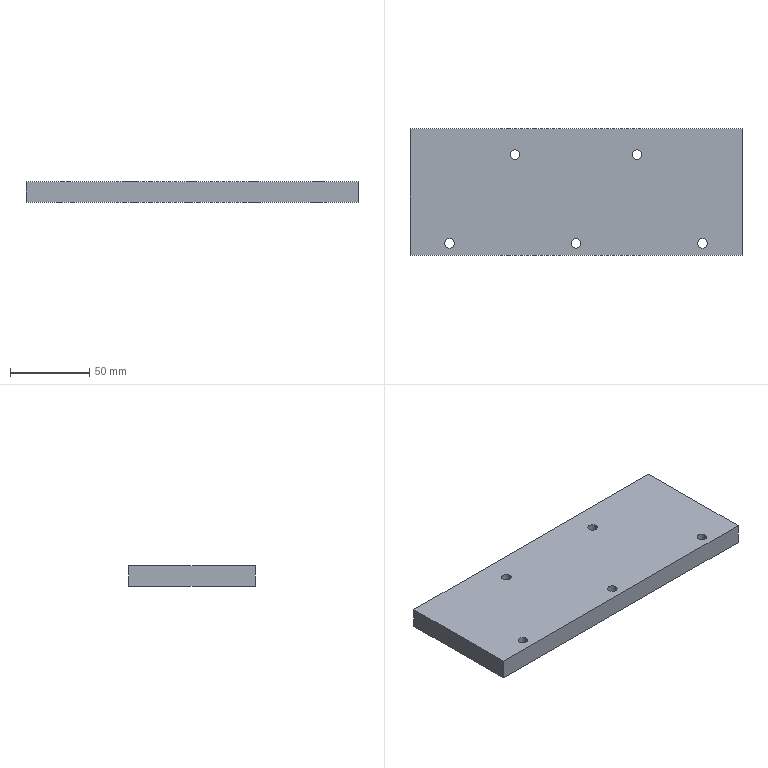Part | SolidWorks | features Cut 4, 3DProfileFeature 2, HoleWzd 2, Extrusion 1 | 1 solid | 39 faces | box 210 x 80 x 13 mm | volume 214445 mm3 | cylinder 24 | plane 11 | cone 4 | commonest cylinder face diameters 6 x10 10 x10 5 x4
STEP:
#1=CARTESIAN_POINT('',(90.,28.,9.));
#2=VERTEX_POINT('',#1);
#3=CARTESIAN_POINT('',(90.,28.,4.));
#4=VERTEX_POINT('',#3);
#5=CARTESIAN_POINT('',(90.,28.,6.5));
#6=DIRECTION('',(1.,0.,0.));
#7=DIRECTION('',(0.,0.,-1.));
#8=AXIS2_PLACEMENT_3D('',#5,#6,#7);
#9=CIRCLE('',#8,2.5);
#10=EDGE_CURVE('',#2,#4,#9,.T.);
#11=ORIENTED_EDGE('',*,*,#10,.F.);
#12=CARTESIAN_POINT('',(105.,28.,9.));
#13=VERTEX_POINT('',#12);
#14=CARTESIAN_POINT('',(105.,28.,9.));
#15=DIRECTION('',(1.,0.,0.));
#16=VECTOR('',#15,1000.);
#17=LINE('',#14,#16);
#18=EDGE_CURVE('',#2,#13,#17,.T.);
#19=ORIENTED_EDGE('',*,*,#18,.T.);
#20=CARTESIAN_POINT('',(105.,28.,4.));
#21=VERTEX_POINT('',#20);
#22=CARTESIAN_POINT('',(105.,28.,6.5));
#23=DIRECTION('',(1.,0.,0.));
#24=DIRECTION('',(0.,0.,-1.));
#25=AXIS2_PLACEMENT_3D('',#22,#23,#24);
#26=CIRCLE('',#25,2.5);
#27=EDGE_CURVE('',#13,#21,#26,.T.);
#28=ORIENTED_EDGE('',*,*,#27,.T.);
#29=CARTESIAN_POINT('',(105.,28.,4.));
#30=DIRECTION('',(1.,0.,0.));
#31=VECTOR('',#30,1000.);
#32=LINE('',#29,#31);
#33=EDGE_CURVE('',#4,#21,#32,.T.);
#34=ORIENTED_EDGE('',*,*,#33,.F.);
#35=EDGE_LOOP('',(#11,#19,#28,#34));
#36=FACE_OUTER_BOUND('',#35,.T.);
#37=CARTESIAN_POINT('',(105.,28.,6.5));
#38=DIRECTION('',(1.,0.,0.));
#39=DIRECTION('',(0.,0.,-1.));
#40=AXIS2_PLACEMENT_3D('',#37,#38,#39);
#41=CYLINDRICAL_SURFACE('',#40,2.5);
#42=ADVANCED_FACE('',(#36),#41,.F.);
#43=CARTESIAN_POINT('',(88.498,28.,6.5));
#44=VERTEX_POINT('',#43);
#45=CARTESIAN_POINT('',(90.,28.,4.));
#46=DIRECTION('',(0.515,0.,-0.8572));
#47=VECTOR('',#46,1000.);
#48=LINE('',#45,#47);
#49=EDGE_CURVE('',#44,#4,#48,.T.);
#50=ORIENTED_EDGE('',*,*,#49,.F.);
#51=CARTESIAN_POINT('',(90.,28.,9.));
#52=DIRECTION('',(0.515,0.,0.8572));
#53=VECTOR('',#52,1000.);
#54=LINE('',#51,#53);
#55=EDGE_CURVE('',#44,#2,#54,.T.);
#56=ORIENTED_EDGE('',*,*,#55,.T.);
#57=ORIENTED_EDGE('',*,*,#10,.T.);
#58=EDGE_LOOP('',(#50,#56,#57));
#59=FACE_OUTER_BOUND('',#58,.T.);
#60=CARTESIAN_POINT('',(90.,28.,6.5));
#61=DIRECTION('',(1.,0.,0.));
#62=DIRECTION('',(0.,0.,-1.));
#63=AXIS2_PLACEMENT_3D('',#60,#61,#62);
#64=CONICAL_SURFACE('',#63,2.5,1.03);
#65=ADVANCED_FACE('',(#59),#64,.F.);
#66=CARTESIAN_POINT('',(-83.,-32.5,13.));
#67=VERTEX_POINT('',#66);
#68=CARTESIAN_POINT('',(-77.,-32.5,13.));
#69=VERTEX_POINT('',#68);
#70=CARTESIAN_POINT('',(-80.,-32.5,13.));
#71=DIRECTION('',(0.,0.,1.));
#72=DIRECTION('',(-1.,0.,0.));
#73=AXIS2_PLACEMENT_3D('',#70,#71,#72);
#74=CIRCLE('',#73,3.);
#75=EDGE_CURVE('',#67,#69,#74,.T.);
#76=ORIENTED_EDGE('',*,*,#75,.T.);
#77=CARTESIAN_POINT('',(-77.,-32.5,6.));
#78=VERTEX_POINT('',#77);
#79=CARTESIAN_POINT('',(-77.,-32.5,13.001));
#80=DIRECTION('',(0.,0.,-1.));
#81=VECTOR('',#80,1000.);
#82=LINE('',#79,#81);
#83=EDGE_CURVE('',#69,#78,#82,.T.);
#84=ORIENTED_EDGE('',*,*,#83,.T.);
#85=CARTESIAN_POINT('',(-83.,-32.5,6.));
#86=VERTEX_POINT('',#85);
#87=CARTESIAN_POINT('',(-80.,-32.5,6.));
#88=DIRECTION('',(0.,0.,1.));
#89=DIRECTION('',(-1.,0.,0.));
#90=AXIS2_PLACEMENT_3D('',#87,#88,#89);
#91=CIRCLE('',#90,3.);
#92=EDGE_CURVE('',#86,#78,#91,.T.);
#93=ORIENTED_EDGE('',*,*,#92,.F.);
#94=CARTESIAN_POINT('',(-83.,-32.5,13.001));
#95=DIRECTION('',(0.,0.,-1.));
#96=VECTOR('',#95,1000.);
#97=LINE('',#94,#96);
#98=EDGE_CURVE('',#67,#86,#97,.T.);
#99=ORIENTED_EDGE('',*,*,#98,.F.);
#100=EDGE_LOOP('',(#76,#84,#93,#99));
#101=FACE_OUTER_BOUND('',#100,.T.);
#102=CARTESIAN_POINT('',(-80.,-32.5,13.001));
#103=DIRECTION('',(0.,0.,-1.));
#104=DIRECTION('',(-1.,0.,0.));
#105=AXIS2_PLACEMENT_3D('',#102,#103,#104);
#106=CYLINDRICAL_SURFACE('',#105,3.);
#107=ADVANCED_FACE('',(#101),#106,.F.);
#108=CARTESIAN_POINT('',(-3.,-32.5,13.));
#109=VERTEX_POINT('',#108);
#110=CARTESIAN_POINT('',(3.,-32.5,13.));
#111=VERTEX_POINT('',#110);
#112=CARTESIAN_POINT('',(0.,-32.5,13.));
#113=DIRECTION('',(0.,0.,1.));
#114=DIRECTION('',(-1.,0.,0.));
#115=AXIS2_PLACEMENT_3D('',#112,#113,#114);
#116=CIRCLE('',#115,3.);
#117=EDGE_CURVE('',#109,#111,#116,.T.);
#118=ORIENTED_EDGE('',*,*,#117,.T.);
#119=CARTESIAN_POINT('',(3.,-32.5,6.));
#120=VERTEX_POINT('',#119);
#121=CARTESIAN_POINT('',(3.,-32.5,13.001));
#122=DIRECTION('',(0.,0.,-1.));
#123=VECTOR('',#122,1000.);
#124=LINE('',#121,#123);
#125=EDGE_CURVE('',#111,#120,#124,.T.);
#126=ORIENTED_EDGE('',*,*,#125,.T.);
#127=CARTESIAN_POINT('',(-3.,-32.5,6.));
#128=VERTEX_POINT('',#127);
#129=CARTESIAN_POINT('',(0.,-32.5,6.));
#130=DIRECTION('',(0.,0.,1.));
#131=DIRECTION('',(-1.,0.,0.));
#132=AXIS2_PLACEMENT_3D('',#129,#130,#131);
#133=CIRCLE('',#132,3.);
#134=EDGE_CURVE('',#128,#120,#133,.T.);
#135=ORIENTED_EDGE('',*,*,#134,.F.);
#136=CARTESIAN_POINT('',(-3.,-32.5,13.001));
#137=DIRECTION('',(0.,0.,-1.));
#138=VECTOR('',#137,1000.);
#139=LINE('',#136,#138);
#140=EDGE_CURVE('',#109,#128,#139,.T.);
#141=ORIENTED_EDGE('',*,*,#140,.F.);
#142=EDGE_LOOP('',(#118,#126,#135,#141));
#143=FACE_OUTER_BOUND('',#142,.T.);
#144=CARTESIAN_POINT('',(0.,-32.5,13.001));
#145=DIRECTION('',(0.,0.,-1.));
#146=DIRECTION('',(-1.,0.,0.));
#147=AXIS2_PLACEMENT_3D('',#144,#145,#146);
#148=CYLINDRICAL_SURFACE('',#147,3.);
#149=ADVANCED_FACE('',(#143),#148,.F.);
#150=CARTESIAN_POINT('',(77.,-32.5,13.));
#151=VERTEX_POINT('',#150);
#152=CARTESIAN_POINT('',(83.,-32.5,13.));
#153=VERTEX_POINT('',#152);
#154=CARTESIAN_POINT('',(80.,-32.5,13.));
#155=DIRECTION('',(0.,0.,1.));
#156=DIRECTION('',(-1.,0.,0.));
#157=AXIS2_PLACEMENT_3D('',#154,#155,#156);
#158=CIRCLE('',#157,3.);
#159=EDGE_CURVE('',#151,#153,#158,.T.);
#160=ORIENTED_EDGE('',*,*,#159,.T.);
#161=CARTESIAN_POINT('',(83.,-32.5,6.));
#162=VERTEX_POINT('',#161);
#163=CARTESIAN_POINT('',(83.,-32.5,13.001));
#164=DIRECTION('',(0.,0.,-1.));
#165=VECTOR('',#164,1000.);
#166=LINE('',#163,#165);
#167=EDGE_CURVE('',#153,#162,#166,.T.);
#168=ORIENTED_EDGE('',*,*,#167,.T.);
#169=CARTESIAN_POINT('',(77.,-32.5,6.));
#170=VERTEX_POINT('',#169);
#171=CARTESIAN_POINT('',(80.,-32.5,6.));
#172=DIRECTION('',(0.,0.,1.));
#173=DIRECTION('',(-1.,0.,0.));
#174=AXIS2_PLACEMENT_3D('',#171,#172,#173);
#175=CIRCLE('',#174,3.);
#176=EDGE_CURVE('',#170,#162,#175,.T.);
#177=ORIENTED_EDGE('',*,*,#176,.F.);
#178=CARTESIAN_POINT('',(77.,-32.5,13.001));
#179=DIRECTION('',(0.,0.,-1.));
#180=VECTOR('',#179,1000.);
#181=LINE('',#178,#180);
#182=EDGE_CURVE('',#151,#170,#181,.T.);
#183=ORIENTED_EDGE('',*,*,#182,.F.);
#184=EDGE_LOOP('',(#160,#168,#177,#183));
#185=FACE_OUTER_BOUND('',#184,.T.);
#186=CARTESIAN_POINT('',(80.,-32.5,13.001));
#187=DIRECTION('',(0.,0.,-1.));
#188=DIRECTION('',(-1.,0.,0.));
#189=AXIS2_PLACEMENT_3D('',#186,#187,#188);
#190=CYLINDRICAL_SURFACE('',#189,3.);
#191=ADVANCED_FACE('',(#185),#190,.F.);
#192=CARTESIAN_POINT('',(5.,-32.5,6.));
#193=VERTEX_POINT('',#192);
#194=CARTESIAN_POINT('',(-5.,-32.5,6.));
#195=VERTEX_POINT('',#194);
#196=CARTESIAN_POINT('',(0.,-32.5,6.));
#197=DIRECTION('',(0.,0.,-1.));
#198=DIRECTION('',(-1.,0.,0.));
#199=AXIS2_PLACEMENT_3D('',#196,#197,#198);
#200=CIRCLE('',#199,5.);
#201=EDGE_CURVE('',#193,#195,#200,.T.);
#202=ORIENTED_EDGE('',*,*,#201,.F.);
#203=CARTESIAN_POINT('',(5.,-32.5,0.));
#204=VERTEX_POINT('',#203);
#205=CARTESIAN_POINT('',(5.,-32.5,6.));
#206=DIRECTION('',(0.,0.,-1.));
#207=VECTOR('',#206,1000.);
#208=LINE('',#205,#207);
#209=EDGE_CURVE('',#193,#204,#208,.T.);
#210=ORIENTED_EDGE('',*,*,#209,.T.);
#211=CARTESIAN_POINT('',(-5.,-32.5,0.));
#212=VERTEX_POINT('',#211);
#213=CARTESIAN_POINT('',(0.,-32.5,0.));
#214=DIRECTION('',(0.,0.,-1.));
#215=DIRECTION('',(-1.,0.,0.));
#216=AXIS2_PLACEMENT_3D('',#213,#214,#215);
#217=CIRCLE('',#216,5.);
#218=EDGE_CURVE('',#204,#212,#217,.T.);
#219=ORIENTED_EDGE('',*,*,#218,.T.);
#220=CARTESIAN_POINT('',(-5.,-32.5,6.));
#221=DIRECTION('',(0.,0.,-1.));
#222=VECTOR('',#221,1000.);
#223=LINE('',#220,#222);
#224=EDGE_CURVE('',#195,#212,#223,.T.);
#225=ORIENTED_EDGE('',*,*,#224,.F.);
#226=EDGE_LOOP('',(#202,#210,#219,#225));
#227=FACE_OUTER_BOUND('',#226,.T.);
#228=CARTESIAN_POINT('',(0.,-32.5,6.));
#229=DIRECTION('',(0.,0.,-1.));
#230=DIRECTION('',(-1.,0.,0.));
#231=AXIS2_PLACEMENT_3D('',#228,#229,#230);
#232=CYLINDRICAL_SURFACE('',#231,5.);
#233=ADVANCED_FACE('',(#227),#232,.F.);
#234=CARTESIAN_POINT('',(-75.,-32.5,6.));
#235=VERTEX_POINT('',#234);
#236=CARTESIAN_POINT('',(-85.,-32.5,6.));
#237=VERTEX_POINT('',#236);
#238=CARTESIAN_POINT('',(-80.,-32.5,6.));
#239=DIRECTION('',(0.,0.,-1.));
#240=DIRECTION('',(-1.,0.,0.));
#241=AXIS2_PLACEMENT_3D('',#238,#239,#240);
#242=CIRCLE('',#241,5.);
#243=EDGE_CURVE('',#235,#237,#242,.T.);
#244=ORIENTED_EDGE('',*,*,#243,.F.);
#245=CARTESIAN_POINT('',(-75.,-32.5,0.));
#246=VERTEX_POINT('',#245);
#247=CARTESIAN_POINT('',(-75.,-32.5,6.));
#248=DIRECTION('',(0.,0.,-1.));
#249=VECTOR('',#248,1000.);
#250=LINE('',#247,#249);
#251=EDGE_CURVE('',#235,#246,#250,.T.);
#252=ORIENTED_EDGE('',*,*,#251,.T.);
#253=CARTESIAN_POINT('',(-85.,-32.5,0.));
#254=VERTEX_POINT('',#253);
#255=CARTESIAN_POINT('',(-80.,-32.5,0.));
#256=DIRECTION('',(0.,0.,-1.));
#257=DIRECTION('',(-1.,0.,0.));
#258=AXIS2_PLACEMENT_3D('',#255,#256,#257);
#259=CIRCLE('',#258,5.);
#260=EDGE_CURVE('',#246,#254,#259,.T.);
#261=ORIENTED_EDGE('',*,*,#260,.T.);
#262=CARTESIAN_POINT('',(-85.,-32.5,6.));
#263=DIRECTION('',(0.,0.,-1.));
#264=VECTOR('',#263,1000.);
#265=LINE('',#262,#264);
#266=EDGE_CURVE('',#237,#254,#265,.T.);
#267=ORIENTED_EDGE('',*,*,#266,.F.);
#268=EDGE_LOOP('',(#244,#252,#261,#267));
#269=FACE_OUTER_BOUND('',#268,.T.);
#270=CARTESIAN_POINT('',(-80.,-32.5,6.));
#271=DIRECTION('',(0.,0.,-1.));
#272=DIRECTION('',(-1.,0.,0.));
#273=AXIS2_PLACEMENT_3D('',#270,#271,#272);
#274=CYLINDRICAL_SURFACE('',#273,5.);
#275=ADVANCED_FACE('',(#269),#274,.F.);
#276=CARTESIAN_POINT('',(85.,-32.5,6.));
#277=VERTEX_POINT('',#276);
#278=CARTESIAN_POINT('',(75.,-32.5,6.));
#279=VERTEX_POINT('',#278);
#280=CARTESIAN_POINT('',(80.,-32.5,6.));
#281=DIRECTION('',(0.,0.,-1.));
#282=DIRECTION('',(-1.,0.,0.));
#283=AXIS2_PLACEMENT_3D('',#280,#281,#282);
#284=CIRCLE('',#283,5.);
#285=EDGE_CURVE('',#277,#279,#284,.T.);
#286=ORIENTED_EDGE('',*,*,#285,.F.);
#287=CARTESIAN_POINT('',(85.,-32.5,0.));
#288=VERTEX_POINT('',#287);
#289=CARTESIAN_POINT('',(85.,-32.5,6.));
#290=DIRECTION('',(0.,0.,-1.));
#291=VECTOR('',#290,1000.);
#292=LINE('',#289,#291);
#293=EDGE_CURVE('',#277,#288,#292,.T.);
#294=ORIENTED_EDGE('',*,*,#293,.T.);
#295=CARTESIAN_POINT('',(75.,-32.5,0.));
#296=VERTEX_POINT('',#295);
#297=CARTESIAN_POINT('',(80.,-32.5,0.));
#298=DIRECTION('',(0.,0.,-1.));
#299=DIRECTION('',(-1.,0.,0.));
#300=AXIS2_PLACEMENT_3D('',#297,#298,#299);
#301=CIRCLE('',#300,5.);
#302=EDGE_CURVE('',#288,#296,#301,.T.);
#303=ORIENTED_EDGE('',*,*,#302,.T.);
#304=CARTESIAN_POINT('',(75.,-32.5,6.));
#305=DIRECTION('',(0.,0.,-1.));
#306=VECTOR('',#305,1000.);
#307=LINE('',#304,#306);
#308=EDGE_CURVE('',#279,#296,#307,.T.);
#309=ORIENTED_EDGE('',*,*,#308,.F.);
#310=EDGE_LOOP('',(#286,#294,#303,#309));
#311=FACE_OUTER_BOUND('',#310,.T.);
#312=CARTESIAN_POINT('',(80.,-32.5,6.));
#313=DIRECTION('',(0.,0.,-1.));
#314=DIRECTION('',(-1.,0.,0.));
#315=AXIS2_PLACEMENT_3D('',#312,#313,#314);
#316=CYLINDRICAL_SURFACE('',#315,5.);
#317=ADVANCED_FACE('',(#311),#316,.F.);
#318=CARTESIAN_POINT('',(90.,-32.5,9.));
#319=VERTEX_POINT('',#318);
#320=CARTESIAN_POINT('',(90.,-32.5,4.));
#321=VERTEX_POINT('',#320);
#322=CARTESIAN_POINT('',(90.,-32.5,6.5));
#323=DIRECTION('',(1.,0.,0.));
#324=DIRECTION('',(0.,0.,-1.));
#325=AXIS2_PLACEMENT_3D('',#322,#323,#324);
#326=CIRCLE('',#325,2.5);
#327=EDGE_CURVE('',#319,#321,#326,.T.);
#328=ORIENTED_EDGE('',*,*,#327,.F.);
#329=CARTESIAN_POINT('',(105.,-32.5,9.));
#330=VERTEX_POINT('',#329);
#331=CARTESIAN_POINT('',(105.,-32.5,9.));
#332=DIRECTION('',(1.,0.,0.));
#333=VECTOR('',#332,1000.);
#334=LINE('',#331,#333);
#335=EDGE_CURVE('',#319,#330,#334,.T.);
#336=ORIENTED_EDGE('',*,*,#335,.T.);
#337=CARTESIAN_POINT('',(105.,-32.5,4.));
#338=VERTEX_POINT('',#337);
#339=CARTESIAN_POINT('',(105.,-32.5,6.5));
#340=DIRECTION('',(1.,0.,0.));
#341=DIRECTION('',(0.,0.,-1.));
#342=AXIS2_PLACEMENT_3D('',#339,#340,#341);
#343=CIRCLE('',#342,2.5);
#344=EDGE_CURVE('',#330,#338,#343,.T.);
#345=ORIENTED_EDGE('',*,*,#344,.T.);
#346=CARTESIAN_POINT('',(105.,-32.5,4.));
#347=DIRECTION('',(1.,0.,0.));
#348=VECTOR('',#347,1000.);
#349=LINE('',#346,#348);
#350=EDGE_CURVE('',#321,#338,#349,.T.);
#351=ORIENTED_EDGE('',*,*,#350,.F.);
#352=EDGE_LOOP('',(#328,#336,#345,#351));
#353=FACE_OUTER_BOUND('',#352,.T.);
#354=CARTESIAN_POINT('',(105.,-32.5,6.5));
#355=DIRECTION('',(1.,0.,0.));
#356=DIRECTION('',(0.,0.,-1.));
#357=AXIS2_PLACEMENT_3D('',#354,#355,#356);
#358=CYLINDRICAL_SURFACE('',#357,2.5);
#359=ADVANCED_FACE('',(#353),#358,.F.);
#360=CARTESIAN_POINT('',(88.498,-32.5,6.5));
#361=VERTEX_POINT('',#360);
#362=CARTESIAN_POINT('',(90.,-32.5,4.));
#363=DIRECTION('',(0.515,0.,-0.8572));
#364=VECTOR('',#363,1000.);
#365=LINE('',#362,#364);
#366=EDGE_CURVE('',#361,#321,#365,.T.);
#367=ORIENTED_EDGE('',*,*,#366,.F.);
#368=CARTESIAN_POINT('',(90.,-32.5,9.));
#369=DIRECTION('',(0.515,0.,0.8572));
#370=VECTOR('',#369,1000.);
#371=LINE('',#368,#370);
#372=EDGE_CURVE('',#361,#319,#371,.T.);
#373=ORIENTED_EDGE('',*,*,#372,.T.);
#374=ORIENTED_EDGE('',*,*,#327,.T.);
#375=EDGE_LOOP('',(#367,#373,#374));
#376=FACE_OUTER_BOUND('',#375,.T.);
#377=CARTESIAN_POINT('',(90.,-32.5,6.5));
#378=DIRECTION('',(1.,0.,0.));
#379=DIRECTION('',(0.,0.,-1.));
#380=AXIS2_PLACEMENT_3D('',#377,#378,#379);
#381=CONICAL_SURFACE('',#380,2.5,1.03);
#382=ADVANCED_FACE('',(#376),#381,.F.);
#383=CARTESIAN_POINT('',(-41.548,23.617,13.));
#384=VERTEX_POINT('',#383);
#385=CARTESIAN_POINT('',(-35.548,23.617,13.));
#386=VERTEX_POINT('',#385);
#387=CARTESIAN_POINT('',(-38.548,23.617,13.));
#388=DIRECTION('',(0.,0.,1.));
#389=DIRECTION('',(-1.,0.,0.));
#390=AXIS2_PLACEMENT_3D('',#387,#388,#389);
#391=CIRCLE('',#390,3.);
#392=EDGE_CURVE('',#384,#386,#391,.T.);
#393=ORIENTED_EDGE('',*,*,#392,.T.);
#394=CARTESIAN_POINT('',(-35.548,23.617,6.));
#395=VERTEX_POINT('',#394);
#396=CARTESIAN_POINT('',(-35.548,23.617,13.001));
#397=DIRECTION('',(0.,0.,-1.));
#398=VECTOR('',#397,1000.);
#399=LINE('',#396,#398);
#400=EDGE_CURVE('',#386,#395,#399,.T.);
#401=ORIENTED_EDGE('',*,*,#400,.T.);
#402=CARTESIAN_POINT('',(-41.548,23.617,6.));
#403=VERTEX_POINT('',#402);
#404=CARTESIAN_POINT('',(-38.548,23.617,6.));
#405=DIRECTION('',(0.,0.,1.));
#406=DIRECTION('',(-1.,0.,0.));
#407=AXIS2_PLACEMENT_3D('',#404,#405,#406);
#408=CIRCLE('',#407,3.);
#409=EDGE_CURVE('',#403,#395,#408,.T.);
#410=ORIENTED_EDGE('',*,*,#409,.F.);
#411=CARTESIAN_POINT('',(-41.548,23.617,13.001));
#412=DIRECTION('',(0.,0.,-1.));
#413=VECTOR('',#412,1000.);
#414=LINE('',#411,#413);
#415=EDGE_CURVE('',#384,#403,#414,.T.);
#416=ORIENTED_EDGE('',*,*,#415,.F.);
#417=EDGE_LOOP('',(#393,#401,#410,#416));
#418=FACE_OUTER_BOUND('',#417,.T.);
#419=CARTESIAN_POINT('',(-38.548,23.617,13.001));
#420=DIRECTION('',(0.,0.,-1.));
#421=DIRECTION('',(-1.,0.,0.));
#422=AXIS2_PLACEMENT_3D('',#419,#420,#421);
#423=CYLINDRICAL_SURFACE('',#422,3.);
#424=ADVANCED_FACE('',(#418),#423,.F.);
#425=CARTESIAN_POINT('',(35.524,23.617,13.));
#426=VERTEX_POINT('',#425);
#427=CARTESIAN_POINT('',(41.524,23.617,13.));
#428=VERTEX_POINT('',#427);
#429=CARTESIAN_POINT('',(38.524,23.617,13.));
#430=DIRECTION('',(0.,0.,1.));
#431=DIRECTION('',(-1.,0.,0.));
#432=AXIS2_PLACEMENT_3D('',#429,#430,#431);
#433=CIRCLE('',#432,3.);
#434=EDGE_CURVE('',#426,#428,#433,.T.);
#435=ORIENTED_EDGE('',*,*,#434,.T.);
#436=CARTESIAN_POINT('',(41.524,23.617,6.));
#437=VERTEX_POINT('',#436);
#438=CARTESIAN_POINT('',(41.524,23.617,13.001));
#439=DIRECTION('',(0.,0.,-1.));
#440=VECTOR('',#439,1000.);
#441=LINE('',#438,#440);
#442=EDGE_CURVE('',#428,#437,#441,.T.);
#443=ORIENTED_EDGE('',*,*,#442,.T.);
#444=CARTESIAN_POINT('',(35.524,23.617,6.));
#445=VERTEX_POINT('',#444);
#446=CARTESIAN_POINT('',(38.524,23.617,6.));
#447=DIRECTION('',(0.,0.,1.));
#448=DIRECTION('',(-1.,0.,0.));
#449=AXIS2_PLACEMENT_3D('',#446,#447,#448);
#450=CIRCLE('',#449,3.);
#451=EDGE_CURVE('',#445,#437,#450,.T.);
#452=ORIENTED_EDGE('',*,*,#451,.F.);
#453=CARTESIAN_POINT('',(35.524,23.617,13.001));
#454=DIRECTION('',(0.,0.,-1.));
#455=VECTOR('',#454,1000.);
#456=LINE('',#453,#455);
#457=EDGE_CURVE('',#426,#445,#456,.T.);
#458=ORIENTED_EDGE('',*,*,#457,.F.);
#459=EDGE_LOOP('',(#435,#443,#452,#458));
#460=FACE_OUTER_BOUND('',#459,.T.);
#461=CARTESIAN_POINT('',(38.524,23.617,13.001));
#462=DIRECTION('',(0.,0.,-1.));
#463=DIRECTION('',(-1.,0.,0.));
#464=AXIS2_PLACEMENT_3D('',#461,#462,#463);
#465=CYLINDRICAL_SURFACE('',#464,3.);
#466=ADVANCED_FACE('',(#460),#465,.F.);
#467=CARTESIAN_POINT('',(-33.548,23.617,6.));
#468=VERTEX_POINT('',#467);
#469=CARTESIAN_POINT('',(-43.548,23.617,6.));
#470=VERTEX_POINT('',#469);
#471=CARTESIAN_POINT('',(-38.548,23.617,6.));
#472=DIRECTION('',(0.,0.,-1.));
#473=DIRECTION('',(-1.,0.,0.));
#474=AXIS2_PLACEMENT_3D('',#471,#472,#473);
#475=CIRCLE('',#474,5.);
#476=EDGE_CURVE('',#468,#470,#475,.T.);
#477=ORIENTED_EDGE('',*,*,#476,.F.);
#478=CARTESIAN_POINT('',(-33.548,23.617,0.));
#479=VERTEX_POINT('',#478);
#480=CARTESIAN_POINT('',(-33.548,23.617,6.));
#481=DIRECTION('',(0.,0.,-1.));
#482=VECTOR('',#481,1000.);
#483=LINE('',#480,#482);
#484=EDGE_CURVE('',#468,#479,#483,.T.);
#485=ORIENTED_EDGE('',*,*,#484,.T.);
#486=CARTESIAN_POINT('',(-43.548,23.617,0.));
#487=VERTEX_POINT('',#486);
#488=CARTESIAN_POINT('',(-38.548,23.617,0.));
#489=DIRECTION('',(0.,0.,-1.));
#490=DIRECTION('',(-1.,0.,0.));
#491=AXIS2_PLACEMENT_3D('',#488,#489,#490);
#492=CIRCLE('',#491,5.);
#493=EDGE_CURVE('',#479,#487,#492,.T.);
#494=ORIENTED_EDGE('',*,*,#493,.T.);
#495=CARTESIAN_POINT('',(-43.548,23.617,6.));
#496=DIRECTION('',(0.,0.,-1.));
#497=VECTOR('',#496,1000.);
#498=LINE('',#495,#497);
#499=EDGE_CURVE('',#470,#487,#498,.T.);
#500=ORIENTED_EDGE('',*,*,#499,.F.);
#501=EDGE_LOOP('',(#477,#485,#494,#500));
#502=FACE_OUTER_BOUND('',#501,.T.);
#503=CARTESIAN_POINT('',(-38.548,23.617,6.));
#504=DIRECTION('',(0.,0.,-1.));
#505=DIRECTION('',(-1.,0.,0.));
#506=AXIS2_PLACEMENT_3D('',#503,#504,#505);
#507=CYLINDRICAL_SURFACE('',#506,5.);
#508=ADVANCED_FACE('',(#502),#507,.F.);
#509=CARTESIAN_POINT('',(43.524,23.617,6.));
#510=VERTEX_POINT('',#509);
#511=CARTESIAN_POINT('',(33.524,23.617,6.));
#512=VERTEX_POINT('',#511);
#513=CARTESIAN_POINT('',(38.524,23.617,6.));
#514=DIRECTION('',(0.,0.,-1.));
#515=DIRECTION('',(-1.,0.,0.));
#516=AXIS2_PLACEMENT_3D('',#513,#514,#515);
#517=CIRCLE('',#516,5.);
#518=EDGE_CURVE('',#510,#512,#517,.T.);
#519=ORIENTED_EDGE('',*,*,#518,.F.);
#520=CARTESIAN_POINT('',(43.524,23.617,0.));
#521=VERTEX_POINT('',#520);
#522=CARTESIAN_POINT('',(43.524,23.617,6.));
#523=DIRECTION('',(0.,0.,-1.));
#524=VECTOR('',#523,1000.);
#525=LINE('',#522,#524);
#526=EDGE_CURVE('',#510,#521,#525,.T.);
#527=ORIENTED_EDGE('',*,*,#526,.T.);
#528=CARTESIAN_POINT('',(33.524,23.617,0.));
#529=VERTEX_POINT('',#528);
#530=CARTESIAN_POINT('',(38.524,23.617,0.));
#531=DIRECTION('',(0.,0.,-1.));
#532=DIRECTION('',(-1.,0.,0.));
#533=AXIS2_PLACEMENT_3D('',#530,#531,#532);
#534=CIRCLE('',#533,5.);
#535=EDGE_CURVE('',#521,#529,#534,.T.);
#536=ORIENTED_EDGE('',*,*,#535,.T.);
#537=CARTESIAN_POINT('',(33.524,23.617,6.));
#538=DIRECTION('',(0.,0.,-1.));
#539=VECTOR('',#538,1000.);
#540=LINE('',#537,#539);
#541=EDGE_CURVE('',#512,#529,#540,.T.);
#542=ORIENTED_EDGE('',*,*,#541,.F.);
#543=EDGE_LOOP('',(#519,#527,#536,#542));
#544=FACE_OUTER_BOUND('',#543,.T.);
#545=CARTESIAN_POINT('',(38.524,23.617,6.));
#546=DIRECTION('',(0.,0.,-1.));
#547=DIRECTION('',(-1.,0.,0.));
#548=AXIS2_PLACEMENT_3D('',#545,#546,#547);
#549=CYLINDRICAL_SURFACE('',#548,5.);
#550=ADVANCED_FACE('',(#544),#549,.F.);
#551=CARTESIAN_POINT('',(105.,28.,6.5));
#552=DIRECTION('',(1.,0.,0.));
#553=DIRECTION('',(0.,0.,-1.));
#554=AXIS2_PLACEMENT_3D('',#551,#552,#553);
#555=CIRCLE('',#554,2.5);
#556=EDGE_CURVE('',#21,#13,#555,.T.);
#557=ORIENTED_EDGE('',*,*,#556,.F.);
#558=ORIENTED_EDGE('',*,*,#27,.F.);
#559=EDGE_LOOP('',(#557,#558));
#560=FACE_BOUND('',#559,.T.);
#561=CARTESIAN_POINT('',(105.,-32.5,6.5));
#562=DIRECTION('',(1.,0.,0.));
#563=DIRECTION('',(0.,0.,-1.));
#564=AXIS2_PLACEMENT_3D('',#561,#562,#563);
#565=CIRCLE('',#564,2.5);
#566=EDGE_CURVE('',#338,#330,#565,.T.);
#567=ORIENTED_EDGE('',*,*,#566,.F.);
#568=ORIENTED_EDGE('',*,*,#344,.F.);
#569=EDGE_LOOP('',(#567,#568));
#570=FACE_BOUND('',#569,.T.);
#571=CARTESIAN_POINT('',(105.,-40.,0.));
#572=VERTEX_POINT('',#571);
#573=CARTESIAN_POINT('',(105.,40.,0.));
#574=VERTEX_POINT('',#573);
#575=CARTESIAN_POINT('',(105.,-40.,0.));
#576=DIRECTION('',(0.,1.,0.));
#577=VECTOR('',#576,1000.);
#578=LINE('',#575,#577);
#579=EDGE_CURVE('',#572,#574,#578,.T.);
#580=ORIENTED_EDGE('',*,*,#579,.T.);
#581=CARTESIAN_POINT('',(105.,40.,13.));
#582=VERTEX_POINT('',#581);
#583=CARTESIAN_POINT('',(105.,40.,13.));
#584=DIRECTION('',(0.,0.,-1.));
#585=VECTOR('',#584,1000.);
#586=LINE('',#583,#585);
#587=EDGE_CURVE('',#582,#574,#586,.T.);
#588=ORIENTED_EDGE('',*,*,#587,.F.);
#589=CARTESIAN_POINT('',(105.,-40.,13.));
#590=VERTEX_POINT('',#589);
#591=CARTESIAN_POINT('',(105.,-40.,13.));
#592=DIRECTION('',(0.,1.,0.));
#593=VECTOR('',#592,1000.);
#594=LINE('',#591,#593);
#595=EDGE_CURVE('',#590,#582,#594,.T.);
#596=ORIENTED_EDGE('',*,*,#595,.F.);
#597=CARTESIAN_POINT('',(105.,-40.,13.));
#598=DIRECTION('',(0.,0.,-1.));
#599=VECTOR('',#598,1000.);
#600=LINE('',#597,#599);
#601=EDGE_CURVE('',#590,#572,#600,.T.);
#602=ORIENTED_EDGE('',*,*,#601,.T.);
#603=EDGE_LOOP('',(#580,#588,#596,#602));
#604=FACE_OUTER_BOUND('',#603,.T.);
#605=CARTESIAN_POINT('',(105.,-40.,13.));
#606=DIRECTION('',(-1.,0.,0.));
#607=DIRECTION('',(0.,0.,1.));
#608=AXIS2_PLACEMENT_3D('',#605,#606,#607);
#609=PLANE('',#608);
#610=ADVANCED_FACE('',(#560,#570,#604),#609,.F.);
#611=CARTESIAN_POINT('',(-105.,40.,0.));
#612=VERTEX_POINT('',#611);
#613=CARTESIAN_POINT('',(-105.,40.,0.));
#614=DIRECTION('',(-1.,0.,0.));
#615=VECTOR('',#614,1000.);
#616=LINE('',#613,#615);
#617=EDGE_CURVE('',#574,#612,#616,.T.);
#618=ORIENTED_EDGE('',*,*,#617,.T.);
#619=CARTESIAN_POINT('',(-105.,40.,13.));
#620=VERTEX_POINT('',#619);
#621=CARTESIAN_POINT('',(-105.,40.,13.));
#622=DIRECTION('',(0.,0.,-1.));
#623=VECTOR('',#622,1000.);
#624=LINE('',#621,#623);
#625=EDGE_CURVE('',#620,#612,#624,.T.);
#626=ORIENTED_EDGE('',*,*,#625,.F.);
#627=CARTESIAN_POINT('',(-105.,40.,13.));
#628=DIRECTION('',(-1.,0.,0.));
#629=VECTOR('',#628,1000.);
#630=LINE('',#627,#629);
#631=EDGE_CURVE('',#582,#620,#630,.T.);
#632=ORIENTED_EDGE('',*,*,#631,.F.);
#633=ORIENTED_EDGE('',*,*,#587,.T.);
#634=EDGE_LOOP('',(#618,#626,#632,#633));
#635=FACE_OUTER_BOUND('',#634,.T.);
#636=CARTESIAN_POINT('',(-105.,40.,13.));
#637=DIRECTION('',(0.,-1.,0.));
#638=DIRECTION('',(0.,0.,-1.));
#639=AXIS2_PLACEMENT_3D('',#636,#637,#638);
#640=PLANE('',#639);
#641=ADVANCED_FACE('',(#635),#640,.F.);
#642=CARTESIAN_POINT('',(-105.,-40.,0.));
#643=VERTEX_POINT('',#642);
#644=CARTESIAN_POINT('',(-105.,-40.,0.));
#645=DIRECTION('',(0.,-1.,0.));
#646=VECTOR('',#645,1000.);
#647=LINE('',#644,#646);
#648=EDGE_CURVE('',#612,#643,#647,.T.);
#649=ORIENTED_EDGE('',*,*,#648,.T.);
#650=CARTESIAN_POINT('',(-105.,-40.,13.));
#651=VERTEX_POINT('',#650);
#652=CARTESIAN_POINT('',(-105.,-40.,13.));
#653=DIRECTION('',(0.,0.,-1.));
#654=VECTOR('',#653,1000.);
#655=LINE('',#652,#654);
#656=EDGE_CURVE('',#651,#643,#655,.T.);
#657=ORIENTED_EDGE('',*,*,#656,.F.);
#658=CARTESIAN_POINT('',(-105.,-40.,13.));
#659=DIRECTION('',(0.,-1.,0.));
#660=VECTOR('',#659,1000.);
#661=LINE('',#658,#660);
#662=EDGE_CURVE('',#620,#651,#661,.T.);
#663=ORIENTED_EDGE('',*,*,#662,.F.);
#664=ORIENTED_EDGE('',*,*,#625,.T.);
#665=EDGE_LOOP('',(#649,#657,#663,#664));
#666=FACE_OUTER_BOUND('',#665,.T.);
#667=CARTESIAN_POINT('',(-105.,-40.,13.));
#668=DIRECTION('',(1.,0.,0.));
#669=DIRECTION('',(0.,0.,-1.));
#670=AXIS2_PLACEMENT_3D('',#667,#668,#669);
#671=PLANE('',#670);
#672=ADVANCED_FACE('',(#666),#671,.F.);
#673=CARTESIAN_POINT('',(-105.,-40.,0.));
#674=DIRECTION('',(1.,0.,0.));
#675=VECTOR('',#674,1000.);
#676=LINE('',#673,#675);
#677=EDGE_CURVE('',#643,#572,#676,.T.);
#678=ORIENTED_EDGE('',*,*,#677,.T.);
#679=ORIENTED_EDGE('',*,*,#601,.F.);
#680=CARTESIAN_POINT('',(-105.,-40.,13.));
#681=DIRECTION('',(1.,0.,0.));
#682=VECTOR('',#681,1000.);
#683=LINE('',#680,#682);
#684=EDGE_CURVE('',#651,#590,#683,.T.);
#685=ORIENTED_EDGE('',*,*,#684,.F.);
#686=ORIENTED_EDGE('',*,*,#656,.T.);
#687=EDGE_LOOP('',(#678,#679,#685,#686));
#688=FACE_OUTER_BOUND('',#687,.T.);
#689=CARTESIAN_POINT('',(-105.,-40.,13.));
#690=DIRECTION('',(0.,1.,0.));
#691=DIRECTION('',(0.,0.,1.));
#692=AXIS2_PLACEMENT_3D('',#689,#690,#691);
#693=PLANE('',#692);
#694=ADVANCED_FACE('',(#688),#693,.F.);
#695=ORIENTED_EDGE('',*,*,#75,.F.);
#696=CARTESIAN_POINT('',(-80.,-32.5,13.));
#697=DIRECTION('',(0.,0.,1.));
#698=DIRECTION('',(-1.,0.,0.));
#699=AXIS2_PLACEMENT_3D('',#696,#697,#698);
#700=CIRCLE('',#699,3.);
#701=EDGE_CURVE('',#69,#67,#700,.T.);
#702=ORIENTED_EDGE('',*,*,#701,.F.);
#703=EDGE_LOOP('',(#695,#702));
#704=FACE_BOUND('',#703,.T.);
#705=ORIENTED_EDGE('',*,*,#117,.F.);
#706=CARTESIAN_POINT('',(0.,-32.5,13.));
#707=DIRECTION('',(0.,0.,1.));
#708=DIRECTION('',(-1.,0.,0.));
#709=AXIS2_PLACEMENT_3D('',#706,#707,#708);
#710=CIRCLE('',#709,3.);
#711=EDGE_CURVE('',#111,#109,#710,.T.);
#712=ORIENTED_EDGE('',*,*,#711,.F.);
#713=EDGE_LOOP('',(#705,#712));
#714=FACE_BOUND('',#713,.T.);
#715=ORIENTED_EDGE('',*,*,#159,.F.);
#716=CARTESIAN_POINT('',(80.,-32.5,13.));
#717=DIRECTION('',(0.,0.,1.));
#718=DIRECTION('',(-1.,0.,0.));
#719=AXIS2_PLACEMENT_3D('',#716,#717,#718);
#720=CIRCLE('',#719,3.);
#721=EDGE_CURVE('',#153,#151,#720,.T.);
#722=ORIENTED_EDGE('',*,*,#721,.F.);
#723=EDGE_LOOP('',(#715,#722));
#724=FACE_BOUND('',#723,.T.);
#725=ORIENTED_EDGE('',*,*,#392,.F.);
#726=CARTESIAN_POINT('',(-38.548,23.617,13.));
#727=DIRECTION('',(0.,0.,1.));
#728=DIRECTION('',(-1.,0.,0.));
#729=AXIS2_PLACEMENT_3D('',#726,#727,#728);
#730=CIRCLE('',#729,3.);
#731=EDGE_CURVE('',#386,#384,#730,.T.);
#732=ORIENTED_EDGE('',*,*,#731,.F.);
#733=EDGE_LOOP('',(#725,#732));
#734=FACE_BOUND('',#733,.T.);
#735=ORIENTED_EDGE('',*,*,#434,.F.);
#736=CARTESIAN_POINT('',(38.524,23.617,13.));
#737=DIRECTION('',(0.,0.,1.));
#738=DIRECTION('',(-1.,0.,0.));
#739=AXIS2_PLACEMENT_3D('',#736,#737,#738);
#740=CIRCLE('',#739,3.);
#741=EDGE_CURVE('',#428,#426,#740,.T.);
#742=ORIENTED_EDGE('',*,*,#741,.F.);
#743=EDGE_LOOP('',(#735,#742));
#744=FACE_BOUND('',#743,.T.);
#745=ORIENTED_EDGE('',*,*,#595,.T.);
#746=ORIENTED_EDGE('',*,*,#631,.T.);
#747=ORIENTED_EDGE('',*,*,#662,.T.);
#748=ORIENTED_EDGE('',*,*,#684,.T.);
#749=EDGE_LOOP('',(#745,#746,#747,#748));
#750=FACE_OUTER_BOUND('',#749,.T.);
#751=CARTESIAN_POINT('',(0.,0.,13.));
#752=DIRECTION('',(0.,0.,-1.));
#753=DIRECTION('',(-1.,0.,0.));
#754=AXIS2_PLACEMENT_3D('',#751,#752,#753);
#755=PLANE('',#754);
#756=ADVANCED_FACE('',(#704,#714,#724,#734,#744,#750),#755,.F.);
#757=CARTESIAN_POINT('',(0.,-32.5,0.));
#758=DIRECTION('',(0.,0.,-1.));
#759=DIRECTION('',(-1.,0.,0.));
#760=AXIS2_PLACEMENT_3D('',#757,#758,#759);
#761=CIRCLE('',#760,5.);
#762=EDGE_CURVE('',#212,#204,#761,.T.);
#763=ORIENTED_EDGE('',*,*,#762,.F.);
#764=ORIENTED_EDGE('',*,*,#218,.F.);
#765=EDGE_LOOP('',(#763,#764));
#766=FACE_BOUND('',#765,.T.);
#767=CARTESIAN_POINT('',(-80.,-32.5,0.));
#768=DIRECTION('',(0.,0.,-1.));
#769=DIRECTION('',(-1.,0.,0.));
#770=AXIS2_PLACEMENT_3D('',#767,#768,#769);
#771=CIRCLE('',#770,5.);
#772=EDGE_CURVE('',#254,#246,#771,.T.);
#773=ORIENTED_EDGE('',*,*,#772,.F.);
#774=ORIENTED_EDGE('',*,*,#260,.F.);
#775=EDGE_LOOP('',(#773,#774));
#776=FACE_BOUND('',#775,.T.);
#777=CARTESIAN_POINT('',(80.,-32.5,0.));
#778=DIRECTION('',(0.,0.,-1.));
#779=DIRECTION('',(-1.,0.,0.));
#780=AXIS2_PLACEMENT_3D('',#777,#778,#779);
#781=CIRCLE('',#780,5.);
#782=EDGE_CURVE('',#296,#288,#781,.T.);
#783=ORIENTED_EDGE('',*,*,#782,.F.);
#784=ORIENTED_EDGE('',*,*,#302,.F.);
#785=EDGE_LOOP('',(#783,#784));
#786=FACE_BOUND('',#785,.T.);
#787=CARTESIAN_POINT('',(-38.548,23.617,0.));
#788=DIRECTION('',(0.,0.,-1.));
#789=DIRECTION('',(-1.,0.,0.));
#790=AXIS2_PLACEMENT_3D('',#787,#788,#789);
#791=CIRCLE('',#790,5.);
#792=EDGE_CURVE('',#487,#479,#791,.T.);
#793=ORIENTED_EDGE('',*,*,#792,.F.);
#794=ORIENTED_EDGE('',*,*,#493,.F.);
#795=EDGE_LOOP('',(#793,#794));
#796=FACE_BOUND('',#795,.T.);
#797=CARTESIAN_POINT('',(38.524,23.617,0.));
#798=DIRECTION('',(0.,0.,-1.));
#799=DIRECTION('',(-1.,0.,0.));
#800=AXIS2_PLACEMENT_3D('',#797,#798,#799);
#801=CIRCLE('',#800,5.);
#802=EDGE_CURVE('',#529,#521,#801,.T.);
#803=ORIENTED_EDGE('',*,*,#802,.F.);
#804=ORIENTED_EDGE('',*,*,#535,.F.);
#805=EDGE_LOOP('',(#803,#804));
#806=FACE_BOUND('',#805,.T.);
#807=ORIENTED_EDGE('',*,*,#579,.F.);
#808=ORIENTED_EDGE('',*,*,#677,.F.);
#809=ORIENTED_EDGE('',*,*,#648,.F.);
#810=ORIENTED_EDGE('',*,*,#617,.F.);
#811=EDGE_LOOP('',(#807,#808,#809,#810));
#812=FACE_OUTER_BOUND('',#811,.T.);
#813=CARTESIAN_POINT('',(0.,0.,0.));
#814=DIRECTION('',(0.,0.,-1.));
#815=DIRECTION('',(-1.,0.,0.));
#816=AXIS2_PLACEMENT_3D('',#813,#814,#815);
#817=PLANE('',#816);
#818=ADVANCED_FACE('',(#766,#776,#786,#796,#806,#812),#817,.T.);
#819=ORIENTED_EDGE('',*,*,#526,.F.);
#820=CARTESIAN_POINT('',(38.524,23.617,6.));
#821=DIRECTION('',(0.,0.,-1.));
#822=DIRECTION('',(-1.,0.,0.));
#823=AXIS2_PLACEMENT_3D('',#820,#821,#822);
#824=CIRCLE('',#823,5.);
#825=EDGE_CURVE('',#512,#510,#824,.T.);
#826=ORIENTED_EDGE('',*,*,#825,.F.);
#827=ORIENTED_EDGE('',*,*,#541,.T.);
#828=ORIENTED_EDGE('',*,*,#802,.T.);
#829=EDGE_LOOP('',(#819,#826,#827,#828));
#830=FACE_OUTER_BOUND('',#829,.T.);
#831=CARTESIAN_POINT('',(38.524,23.617,6.));
#832=DIRECTION('',(0.,0.,-1.));
#833=DIRECTION('',(-1.,0.,0.));
#834=AXIS2_PLACEMENT_3D('',#831,#832,#833);
#835=CYLINDRICAL_SURFACE('',#834,5.);
#836=ADVANCED_FACE('',(#830),#835,.F.);
#837=ORIENTED_EDGE('',*,*,#451,.T.);
#838=CARTESIAN_POINT('',(38.524,23.617,6.));
#839=DIRECTION('',(0.,0.,1.));
#840=DIRECTION('',(-1.,0.,0.));
#841=AXIS2_PLACEMENT_3D('',#838,#839,#840);
#842=CIRCLE('',#841,3.);
#843=EDGE_CURVE('',#437,#445,#842,.T.);
#844=ORIENTED_EDGE('',*,*,#843,.T.);
#845=EDGE_LOOP('',(#837,#844));
#846=FACE_BOUND('',#845,.T.);
#847=ORIENTED_EDGE('',*,*,#825,.T.);
#848=ORIENTED_EDGE('',*,*,#518,.T.);
#849=EDGE_LOOP('',(#847,#848));
#850=FACE_OUTER_BOUND('',#849,.T.);
#851=CARTESIAN_POINT('',(0.,0.,6.));
#852=DIRECTION('',(0.,0.,-1.));
#853=DIRECTION('',(-1.,0.,0.));
#854=AXIS2_PLACEMENT_3D('',#851,#852,#853);
#855=PLANE('',#854);
#856=ADVANCED_FACE('',(#846,#850),#855,.T.);
#857=ORIENTED_EDGE('',*,*,#484,.F.);
#858=CARTESIAN_POINT('',(-38.548,23.617,6.));
#859=DIRECTION('',(0.,0.,-1.));
#860=DIRECTION('',(-1.,0.,0.));
#861=AXIS2_PLACEMENT_3D('',#858,#859,#860);
#862=CIRCLE('',#861,5.);
#863=EDGE_CURVE('',#470,#468,#862,.T.);
#864=ORIENTED_EDGE('',*,*,#863,.F.);
#865=ORIENTED_EDGE('',*,*,#499,.T.);
#866=ORIENTED_EDGE('',*,*,#792,.T.);
#867=EDGE_LOOP('',(#857,#864,#865,#866));
#868=FACE_OUTER_BOUND('',#867,.T.);
#869=CARTESIAN_POINT('',(-38.548,23.617,6.));
#870=DIRECTION('',(0.,0.,-1.));
#871=DIRECTION('',(-1.,0.,0.));
#872=AXIS2_PLACEMENT_3D('',#869,#870,#871);
#873=CYLINDRICAL_SURFACE('',#872,5.);
#874=ADVANCED_FACE('',(#868),#873,.F.);
#875=ORIENTED_EDGE('',*,*,#409,.T.);
#876=CARTESIAN_POINT('',(-38.548,23.617,6.));
#877=DIRECTION('',(0.,0.,1.));
#878=DIRECTION('',(-1.,0.,0.));
#879=AXIS2_PLACEMENT_3D('',#876,#877,#878);
#880=CIRCLE('',#879,3.);
#881=EDGE_CURVE('',#395,#403,#880,.T.);
#882=ORIENTED_EDGE('',*,*,#881,.T.);
#883=EDGE_LOOP('',(#875,#882));
#884=FACE_BOUND('',#883,.T.);
#885=ORIENTED_EDGE('',*,*,#863,.T.);
#886=ORIENTED_EDGE('',*,*,#476,.T.);
#887=EDGE_LOOP('',(#885,#886));
#888=FACE_OUTER_BOUND('',#887,.T.);
#889=CARTESIAN_POINT('',(0.,0.,6.));
#890=DIRECTION('',(0.,0.,-1.));
#891=DIRECTION('',(-1.,0.,0.));
#892=AXIS2_PLACEMENT_3D('',#889,#890,#891);
#893=PLANE('',#892);
#894=ADVANCED_FACE('',(#884,#888),#893,.T.);
#895=ORIENTED_EDGE('',*,*,#442,.F.);
#896=ORIENTED_EDGE('',*,*,#741,.T.);
#897=ORIENTED_EDGE('',*,*,#457,.T.);
#898=ORIENTED_EDGE('',*,*,#843,.F.);
#899=EDGE_LOOP('',(#895,#896,#897,#898));
#900=FACE_OUTER_BOUND('',#899,.T.);
#901=CARTESIAN_POINT('',(38.524,23.617,13.001));
#902=DIRECTION('',(0.,0.,-1.));
#903=DIRECTION('',(-1.,0.,0.));
#904=AXIS2_PLACEMENT_3D('',#901,#902,#903);
#905=CYLINDRICAL_SURFACE('',#904,3.);
#906=ADVANCED_FACE('',(#900),#905,.F.);
#907=ORIENTED_EDGE('',*,*,#400,.F.);
#908=ORIENTED_EDGE('',*,*,#731,.T.);
#909=ORIENTED_EDGE('',*,*,#415,.T.);
#910=ORIENTED_EDGE('',*,*,#881,.F.);
#911=EDGE_LOOP('',(#907,#908,#909,#910));
#912=FACE_OUTER_BOUND('',#911,.T.);
#913=CARTESIAN_POINT('',(-38.548,23.617,13.001));
#914=DIRECTION('',(0.,0.,-1.));
#915=DIRECTION('',(-1.,0.,0.));
#916=AXIS2_PLACEMENT_3D('',#913,#914,#915);
#917=CYLINDRICAL_SURFACE('',#916,3.);
#918=ADVANCED_FACE('',(#912),#917,.F.);
#919=ORIENTED_EDGE('',*,*,#372,.F.);
#920=ORIENTED_EDGE('',*,*,#366,.T.);
#921=CARTESIAN_POINT('',(90.,-32.5,6.5));
#922=DIRECTION('',(1.,0.,0.));
#923=DIRECTION('',(0.,0.,-1.));
#924=AXIS2_PLACEMENT_3D('',#921,#922,#923);
#925=CIRCLE('',#924,2.5);
#926=EDGE_CURVE('',#321,#319,#925,.T.);
#927=ORIENTED_EDGE('',*,*,#926,.T.);
#928=EDGE_LOOP('',(#919,#920,#927));
#929=FACE_OUTER_BOUND('',#928,.T.);
#930=CARTESIAN_POINT('',(90.,-32.5,6.5));
#931=DIRECTION('',(1.,0.,0.));
#932=DIRECTION('',(0.,0.,-1.));
#933=AXIS2_PLACEMENT_3D('',#930,#931,#932);
#934=CONICAL_SURFACE('',#933,2.5,1.03);
#935=ADVANCED_FACE('',(#929),#934,.F.);
#936=ORIENTED_EDGE('',*,*,#335,.F.);
#937=ORIENTED_EDGE('',*,*,#926,.F.);
#938=ORIENTED_EDGE('',*,*,#350,.T.);
#939=ORIENTED_EDGE('',*,*,#566,.T.);
#940=EDGE_LOOP('',(#936,#937,#938,#939));
#941=FACE_OUTER_BOUND('',#940,.T.);
#942=CARTESIAN_POINT('',(105.,-32.5,6.5));
#943=DIRECTION('',(1.,0.,0.));
#944=DIRECTION('',(0.,0.,-1.));
#945=AXIS2_PLACEMENT_3D('',#942,#943,#944);
#946=CYLINDRICAL_SURFACE('',#945,2.5);
#947=ADVANCED_FACE('',(#941),#946,.F.);
#948=ORIENTED_EDGE('',*,*,#293,.F.);
#949=CARTESIAN_POINT('',(80.,-32.5,6.));
#950=DIRECTION('',(0.,0.,-1.));
#951=DIRECTION('',(-1.,0.,0.));
#952=AXIS2_PLACEMENT_3D('',#949,#950,#951);
#953=CIRCLE('',#952,5.);
#954=EDGE_CURVE('',#279,#277,#953,.T.);
#955=ORIENTED_EDGE('',*,*,#954,.F.);
#956=ORIENTED_EDGE('',*,*,#308,.T.);
#957=ORIENTED_EDGE('',*,*,#782,.T.);
#958=EDGE_LOOP('',(#948,#955,#956,#957));
#959=FACE_OUTER_BOUND('',#958,.T.);
#960=CARTESIAN_POINT('',(80.,-32.5,6.));
#961=DIRECTION('',(0.,0.,-1.));
#962=DIRECTION('',(-1.,0.,0.));
#963=AXIS2_PLACEMENT_3D('',#960,#961,#962);
#964=CYLINDRICAL_SURFACE('',#963,5.);
#965=ADVANCED_FACE('',(#959),#964,.F.);
#966=ORIENTED_EDGE('',*,*,#176,.T.);
#967=CARTESIAN_POINT('',(80.,-32.5,6.));
#968=DIRECTION('',(0.,0.,1.));
#969=DIRECTION('',(-1.,0.,0.));
#970=AXIS2_PLACEMENT_3D('',#967,#968,#969);
#971=CIRCLE('',#970,3.);
#972=EDGE_CURVE('',#162,#170,#971,.T.);
#973=ORIENTED_EDGE('',*,*,#972,.T.);
#974=EDGE_LOOP('',(#966,#973));
#975=FACE_BOUND('',#974,.T.);
#976=ORIENTED_EDGE('',*,*,#954,.T.);
#977=ORIENTED_EDGE('',*,*,#285,.T.);
#978=EDGE_LOOP('',(#976,#977));
#979=FACE_OUTER_BOUND('',#978,.T.);
#980=CARTESIAN_POINT('',(0.,0.,6.));
#981=DIRECTION('',(0.,0.,-1.));
#982=DIRECTION('',(-1.,0.,0.));
#983=AXIS2_PLACEMENT_3D('',#980,#981,#982);
#984=PLANE('',#983);
#985=ADVANCED_FACE('',(#975,#979),#984,.T.);
#986=ORIENTED_EDGE('',*,*,#251,.F.);
#987=CARTESIAN_POINT('',(-80.,-32.5,6.));
#988=DIRECTION('',(0.,0.,-1.));
#989=DIRECTION('',(-1.,0.,0.));
#990=AXIS2_PLACEMENT_3D('',#987,#988,#989);
#991=CIRCLE('',#990,5.);
#992=EDGE_CURVE('',#237,#235,#991,.T.);
#993=ORIENTED_EDGE('',*,*,#992,.F.);
#994=ORIENTED_EDGE('',*,*,#266,.T.);
#995=ORIENTED_EDGE('',*,*,#772,.T.);
#996=EDGE_LOOP('',(#986,#993,#994,#995));
#997=FACE_OUTER_BOUND('',#996,.T.);
#998=CARTESIAN_POINT('',(-80.,-32.5,6.));
#999=DIRECTION('',(0.,0.,-1.));
#1000=DIRECTION('',(-1.,0.,0.));
#1001=AXIS2_PLACEMENT_3D('',#998,#999,#1000);
#1002=CYLINDRICAL_SURFACE('',#1001,5.);
#1003=ADVANCED_FACE('',(#997),#1002,.F.);
#1004=ORIENTED_EDGE('',*,*,#92,.T.);
#1005=CARTESIAN_POINT('',(-80.,-32.5,6.));
#1006=DIRECTION('',(0.,0.,1.));
#1007=DIRECTION('',(-1.,0.,0.));
#1008=AXIS2_PLACEMENT_3D('',#1005,#1006,#1007);
#1009=CIRCLE('',#1008,3.);
#1010=EDGE_CURVE('',#78,#86,#1009,.T.);
#1011=ORIENTED_EDGE('',*,*,#1010,.T.);
#1012=EDGE_LOOP('',(#1004,#1011));
#1013=FACE_BOUND('',#1012,.T.);
#1014=ORIENTED_EDGE('',*,*,#992,.T.);
#1015=ORIENTED_EDGE('',*,*,#243,.T.);
#1016=EDGE_LOOP('',(#1014,#1015));
#1017=FACE_OUTER_BOUND('',#1016,.T.);
#1018=CARTESIAN_POINT('',(0.,0.,6.));
#1019=DIRECTION('',(0.,0.,-1.));
#1020=DIRECTION('',(-1.,0.,0.));
#1021=AXIS2_PLACEMENT_3D('',#1018,#1019,#1020);
#1022=PLANE('',#1021);
#1023=ADVANCED_FACE('',(#1013,#1017),#1022,.T.);
#1024=ORIENTED_EDGE('',*,*,#209,.F.);
#1025=CARTESIAN_POINT('',(0.,-32.5,6.));
#1026=DIRECTION('',(0.,0.,-1.));
#1027=DIRECTION('',(-1.,0.,0.));
#1028=AXIS2_PLACEMENT_3D('',#1025,#1026,#1027);
#1029=CIRCLE('',#1028,5.);
#1030=EDGE_CURVE('',#195,#193,#1029,.T.);
#1031=ORIENTED_EDGE('',*,*,#1030,.F.);
#1032=ORIENTED_EDGE('',*,*,#224,.T.);
#1033=ORIENTED_EDGE('',*,*,#762,.T.);
#1034=EDGE_LOOP('',(#1024,#1031,#1032,#1033));
#1035=FACE_OUTER_BOUND('',#1034,.T.);
#1036=CARTESIAN_POINT('',(0.,-32.5,6.));
#1037=DIRECTION('',(0.,0.,-1.));
#1038=DIRECTION('',(-1.,0.,0.));
#1039=AXIS2_PLACEMENT_3D('',#1036,#1037,#1038);
#1040=CYLINDRICAL_SURFACE('',#1039,5.);
#1041=ADVANCED_FACE('',(#1035),#1040,.F.);
#1042=ORIENTED_EDGE('',*,*,#134,.T.);
#1043=CARTESIAN_POINT('',(0.,-32.5,6.));
#1044=DIRECTION('',(0.,0.,1.));
#1045=DIRECTION('',(-1.,0.,0.));
#1046=AXIS2_PLACEMENT_3D('',#1043,#1044,#1045);
#1047=CIRCLE('',#1046,3.);
#1048=EDGE_CURVE('',#120,#128,#1047,.T.);
#1049=ORIENTED_EDGE('',*,*,#1048,.T.);
#1050=EDGE_LOOP('',(#1042,#1049));
#1051=FACE_BOUND('',#1050,.T.);
#1052=ORIENTED_EDGE('',*,*,#1030,.T.);
#1053=ORIENTED_EDGE('',*,*,#201,.T.);
#1054=EDGE_LOOP('',(#1052,#1053));
#1055=FACE_OUTER_BOUND('',#1054,.T.);
#1056=CARTESIAN_POINT('',(0.,0.,6.));
#1057=DIRECTION('',(0.,0.,-1.));
#1058=DIRECTION('',(-1.,0.,0.));
#1059=AXIS2_PLACEMENT_3D('',#1056,#1057,#1058);
#1060=PLANE('',#1059);
#1061=ADVANCED_FACE('',(#1051,#1055),#1060,.T.);
#1062=ORIENTED_EDGE('',*,*,#167,.F.);
#1063=ORIENTED_EDGE('',*,*,#721,.T.);
#1064=ORIENTED_EDGE('',*,*,#182,.T.);
#1065=ORIENTED_EDGE('',*,*,#972,.F.);
#1066=EDGE_LOOP('',(#1062,#1063,#1064,#1065));
#1067=FACE_OUTER_BOUND('',#1066,.T.);
#1068=CARTESIAN_POINT('',(80.,-32.5,13.001));
#1069=DIRECTION('',(0.,0.,-1.));
#1070=DIRECTION('',(-1.,0.,0.));
#1071=AXIS2_PLACEMENT_3D('',#1068,#1069,#1070);
#1072=CYLINDRICAL_SURFACE('',#1071,3.);
#1073=ADVANCED_FACE('',(#1067),#1072,.F.);
#1074=ORIENTED_EDGE('',*,*,#125,.F.);
#1075=ORIENTED_EDGE('',*,*,#711,.T.);
#1076=ORIENTED_EDGE('',*,*,#140,.T.);
#1077=ORIENTED_EDGE('',*,*,#1048,.F.);
#1078=EDGE_LOOP('',(#1074,#1075,#1076,#1077));
#1079=FACE_OUTER_BOUND('',#1078,.T.);
#1080=CARTESIAN_POINT('',(0.,-32.5,13.001));
#1081=DIRECTION('',(0.,0.,-1.));
#1082=DIRECTION('',(-1.,0.,0.));
#1083=AXIS2_PLACEMENT_3D('',#1080,#1081,#1082);
#1084=CYLINDRICAL_SURFACE('',#1083,3.);
#1085=ADVANCED_FACE('',(#1079),#1084,.F.);
#1086=ORIENTED_EDGE('',*,*,#83,.F.);
#1087=ORIENTED_EDGE('',*,*,#701,.T.);
#1088=ORIENTED_EDGE('',*,*,#98,.T.);
#1089=ORIENTED_EDGE('',*,*,#1010,.F.);
#1090=EDGE_LOOP('',(#1086,#1087,#1088,#1089));
#1091=FACE_OUTER_BOUND('',#1090,.T.);
#1092=CARTESIAN_POINT('',(-80.,-32.5,13.001));
#1093=DIRECTION('',(0.,0.,-1.));
#1094=DIRECTION('',(-1.,0.,0.));
#1095=AXIS2_PLACEMENT_3D('',#1092,#1093,#1094);
#1096=CYLINDRICAL_SURFACE('',#1095,3.);
#1097=ADVANCED_FACE('',(#1091),#1096,.F.);
#1098=ORIENTED_EDGE('',*,*,#55,.F.);
#1099=ORIENTED_EDGE('',*,*,#49,.T.);
#1100=CARTESIAN_POINT('',(90.,28.,6.5));
#1101=DIRECTION('',(1.,0.,0.));
#1102=DIRECTION('',(0.,0.,-1.));
#1103=AXIS2_PLACEMENT_3D('',#1100,#1101,#1102);
#1104=CIRCLE('',#1103,2.5);
#1105=EDGE_CURVE('',#4,#2,#1104,.T.);
#1106=ORIENTED_EDGE('',*,*,#1105,.T.);
#1107=EDGE_LOOP('',(#1098,#1099,#1106));
#1108=FACE_OUTER_BOUND('',#1107,.T.);
#1109=CARTESIAN_POINT('',(90.,28.,6.5));
#1110=DIRECTION('',(1.,0.,0.));
#1111=DIRECTION('',(0.,0.,-1.));
#1112=AXIS2_PLACEMENT_3D('',#1109,#1110,#1111);
#1113=CONICAL_SURFACE('',#1112,2.5,1.03);
#1114=ADVANCED_FACE('',(#1108),#1113,.F.);
#1115=ORIENTED_EDGE('',*,*,#18,.F.);
#1116=ORIENTED_EDGE('',*,*,#1105,.F.);
#1117=ORIENTED_EDGE('',*,*,#33,.T.);
#1118=ORIENTED_EDGE('',*,*,#556,.T.);
#1119=EDGE_LOOP('',(#1115,#1116,#1117,#1118));
#1120=FACE_OUTER_BOUND('',#1119,.T.);
#1121=CARTESIAN_POINT('',(105.,28.,6.5));
#1122=DIRECTION('',(1.,0.,0.));
#1123=DIRECTION('',(0.,0.,-1.));
#1124=AXIS2_PLACEMENT_3D('',#1121,#1122,#1123);
#1125=CYLINDRICAL_SURFACE('',#1124,2.5);
#1126=ADVANCED_FACE('',(#1120),#1125,.F.);
#1127=CLOSED_SHELL('',(#42,#65,#107,#149,#191,#233,#275,#317,#359,#382,#424,#466,#508,#550,#610,#641,#672,#694,#756,#818,#836,#856,#874,#894,#906,#918,#935,#947,#965,#985,#1003,#1023,#1041,#1061,#1073,#1085,#1097,#1114,#1126));
#1128=MANIFOLD_SOLID_BREP('',#1127);
#1129=CARTESIAN_POINT('',(0.,0.,0.));
#1130=DIRECTION('',(0.,0.,1.));
#1131=DIRECTION('',(1.,0.,0.));
#1132=AXIS2_PLACEMENT_3D('',#1129,#1130,#1131);
#1133=(LENGTH_UNIT()NAMED_UNIT(*)SI_UNIT(.MILLI.,.METRE.));
#1134=UNCERTAINTY_MEASURE_WITH_UNIT(LENGTH_MEASURE(0.00001),#1133,'','');
#1135=(NAMED_UNIT(*)PLANE_ANGLE_UNIT()SI_UNIT($,.RADIAN.));
#1136=(NAMED_UNIT(*)SI_UNIT($,.STERADIAN.)SOLID_ANGLE_UNIT());
#1137=(GEOMETRIC_REPRESENTATION_CONTEXT(3)GLOBAL_UNCERTAINTY_ASSIGNED_CONTEXT((#1134))GLOBAL_UNIT_ASSIGNED_CONTEXT((#1133,#1135,#1136))REPRESENTATION_CONTEXT('',''));
#1138=ADVANCED_BREP_SHAPE_REPRESENTATION('',(#1128,#1132),#1137);